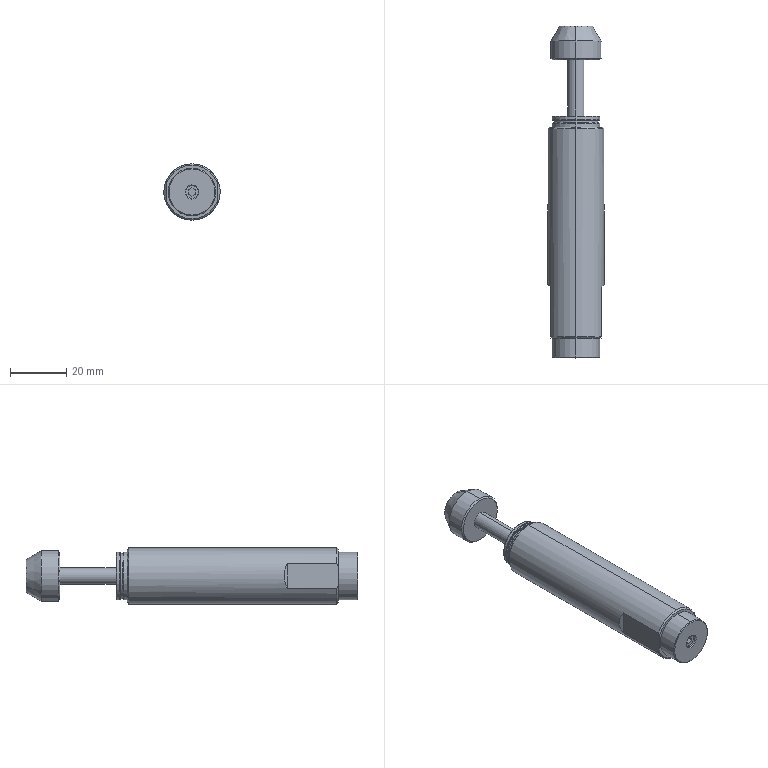Part | STEP file | ACA-2020-3 | 1 solid | 61 faces | box 20 x 118 x 20 mm | volume 28972 mm3 | plane 20 | cone 17 | cylinder 16 | spline 8 | commonest cylinder face diameters 17 x6 4.459 x2 6 x2 16 x2 18 x2 20 x2